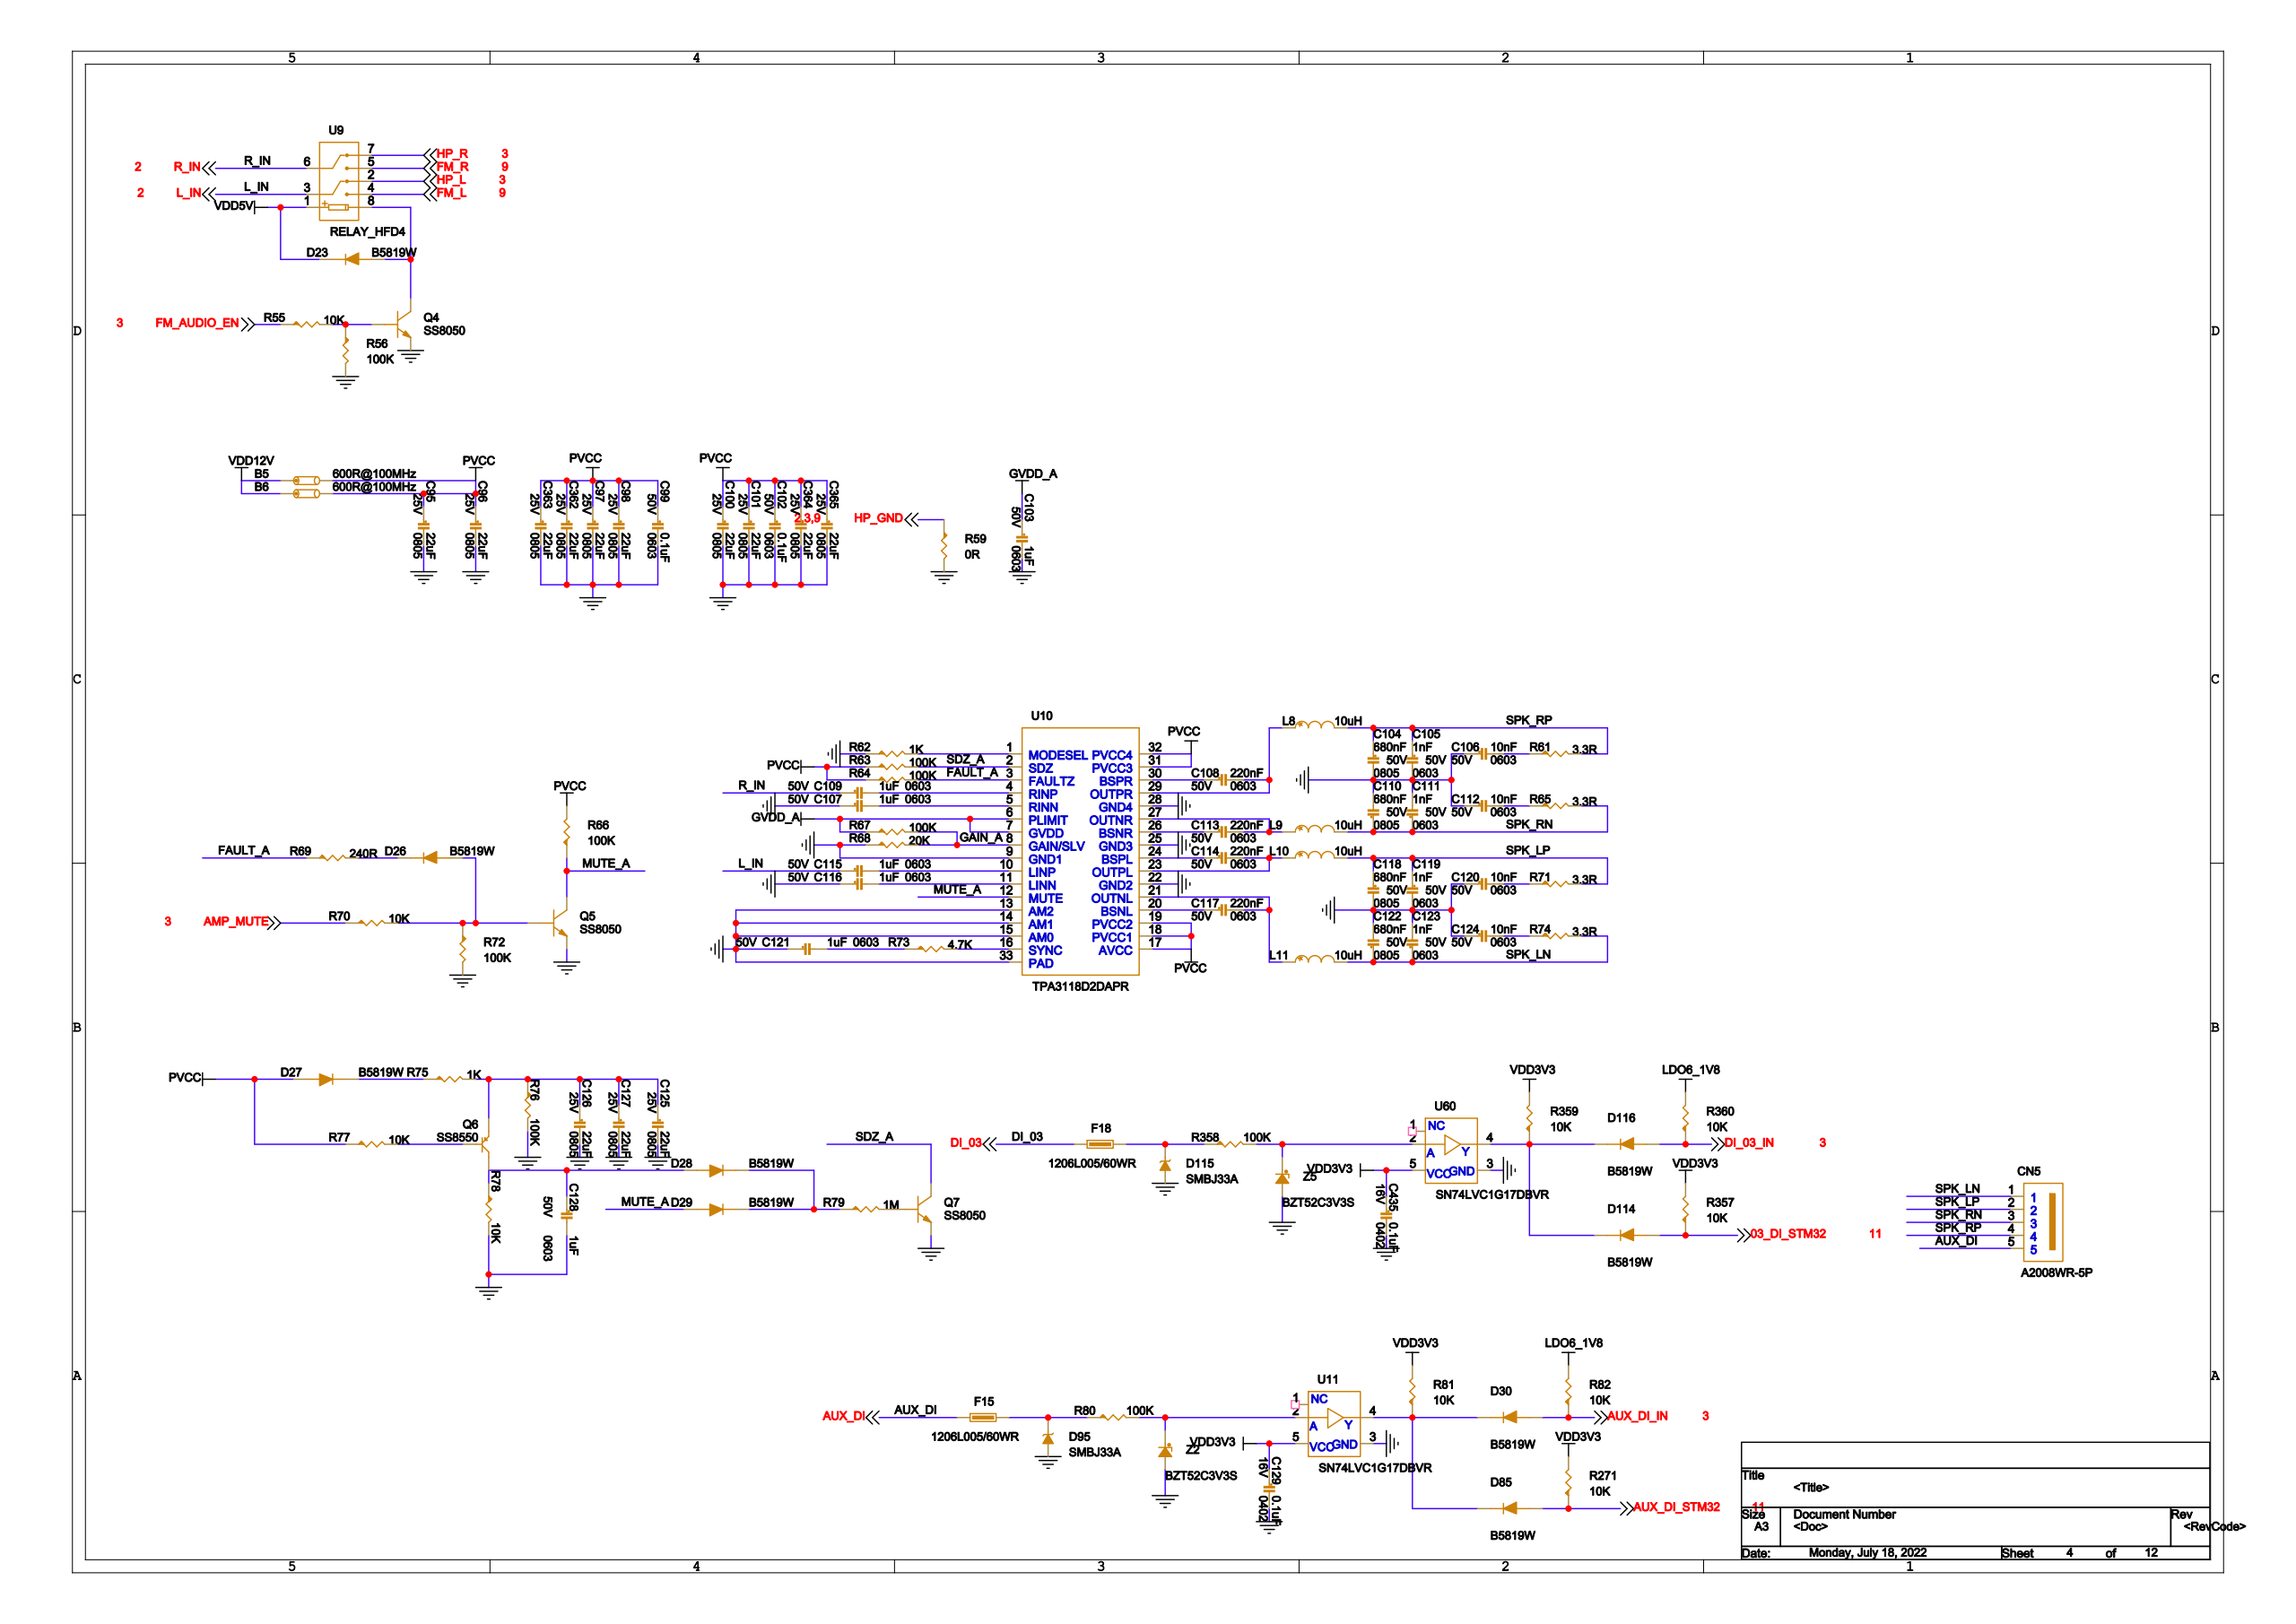Circuit board | Cadence Allegro | 970 parts | 627 nets | one sheet of the schematic
Parts on this sheet (reference | value | footprint):
B5 | 600R@100MHz | R0805
B6 | 600R@100MHz | R0805
C95 | 22uF | C0805
C96 | 22uF | C0805
C97 | 22uF | C0805
C98 | 22uF | C0805
C99 | 0.1uF | C0603
C100 | 22uF | C0805
C101 | 22uF | C0805
C102 | 0.1uF | C0603
C103 | 1uF | C0603
C104 | 680nF | C0805
C105 | 1nF | C0603
C106 | 10nF | C0603
C107 | 1uF | C0603
C108 | 220nF | C0603
C109 | 1uF | C0603
C110 | 680nF | C0805
C111 | 1nF | C0603
C112 | 10nF | C0603
C113 | 220nF | C0603
C114 | 220nF | C0603
C115 | 1uF | C0603
C116 | 1uF | C0603
C117 | 220nF | C0603
C118 | 680nF | C0805
C119 | 1nF | C0603
C120 | 10nF | C0603
C121 | 1uF | C0603
C122 | 680nF | C0805
C123 | 1nF | C0603
C124 | 10nF | C0603
C125 | 22uF | C0805
C126 | 22uF | C0805
C127 | 22uF | C0805
C128 | 1uF | C0603
C129 | 0.1uF | C0402
C362 | 22uF | C0805
C363 | 22uF | C0805
C364 | 22uF | C0805
C365 | 22uF | C0805
C435 | 0.1uF | C0402
CN5 | A2008WR-5P | A2008WR_5P
D23 | B5819W | SOD-123
D26 | B5819W | SOD-123
D27 | B5819W | SOD-123
D28 | B5819W | SOD-123
D29 | B5819W | SOD-123
D30 | B5819W | SOD-123
D85 | B5819W | SOD-123
D95 | SMBJ33A | SMB
D114 | B5819W | SOD-123
D115 | SMBJ33A | SMB
D116 | B5819W | SOD-123
F15 | 1206L005/60WR | R1206
F18 | 1206L005/60WR | R1206
L8 | 10uH | IND0630
L9 | 10uH | IND0630
L10 | 10uH | IND0630
L11 | 10uH | IND0630
Q4 | SS8050 | SOT-23
Q5 | SS8050 | SOT-23
Q6 | SS8550 | SOT-23
Q7 | SS8050 | SOT-23
R55 | 10K | R0402
R56 | 100K | R0402
R59 | 0R | R0402
R61 | 3.3R | R0603
R62 | 1K | R0402
R63 | 100K | R0402
R64 | 100K | R0402
R65 | 3.3R | R0603
R66 | 100K | R0402
R67 | 100K | R0402
R68 | 20K | R0402
R69 | 240R | R0402
R70 | 10K | R0402
R71 | 3.3R | R0603
R72 | 100K | R0402
R73 | 4.7K | R0402
R74 | 3.3R | R0603
R75 | 1K | R0402
R76 | 100K | R0402
R77 | 10K | R0402
R78 | 10K | R0402
R79 | 1M | R0402
R80 | 100K | R0402
R81 | 10K | R0402
R82 | 10K | R0402
R271 | 10K | R0402
R357 | 10K | R0402
R358 | 100K | R0402
R359 | 10K | R0402
R360 | 10K | R0402
U9 | RELAY_HFD4 | RELAY_HFD4
U10 | TPA3118D2DAPR | HTSSOP32
U11 | SN74LVC1G17DBVR | SOT23-5
U60 | SN74LVC1G17DBVR | SOT23-5
Z2 | BZT52C3V3S | SOD323
Z5 | BZT52C3V3S | SOD323
Nets of these parts (net: part-pin ...):
VDD5V: D23-2 U9-1
VDD3V3: C129-1 C435-1 R81-2 R271-2 R357-2 R359-2 U11-5 U60-5
GND: C95-2 C96-2 C97-2 C98-2 C99-2 C100-2 C101-2 C102-2 C103-2 C104-2 C105-2 C106-1 C107-1 C110-2 C111-2 C112-1 C116-1 C118-2 C119-2 C120-1 C121-1 C122-2 C123-2 C124-1 C125-2 C126-2 C127-2 C128-2 C129-2 C362-2 C363-2 C364-2 C365-2 C435-2 D95-1 D115-1 Q4-2 Q5-2 Q7-2 R56-2 R59-2 R62-1 R68-1 R72-2 R76-2 R78-2 U11-3 U60-3 Z2-1 Z5-1 U10-9 U10-13 U10-14 U10-15 U10-22 U10-25 U10-28 U10-33
LDO6_1V8: R82-2 R360-2
SPK_LN: C122-1 C123-1 CN5-1 L11-2 R74-2
SPK_LP: C118-1 C119-1 CN5-2 L10-2 R71-2
SPK_RN: C110-1 C111-1 CN5-3 L9-2 R65-2
SPK_RP: C104-1 C105-1 CN5-4 L8-2 R61-2
AUX_DI: CN5-5 F15-1
VDD12V: B5-1 B6-1
N19779625: D115-2 F18-2 R358-1
N19387563: D95-2 F15-2 R80-1
DI_03: F18-1
N19779643: R358-2 U60-2 Z5-2
N19779563: D114-2 D116-2 R359-1 U60-4
N19387544: R80-2 U11-2 Z2-2
N19387510: D30-2 D85-2 R81-1 U11-4
HP_L: U9-2
HP_GND: R59-1
HP_R: U9-7
N19224261: C106-2 R61-1
N19224258: C112-2 R65-1
N19224400: C120-2 R71-1
N19224398: C124-2 R74-1
N19223689: C108-1 U10-30
N19223692: C108-2 L8-1 U10-29
N19223701: C113-1 U10-26
N19223704: C113-2 L9-1 U10-27
N19223713: C114-1 U10-24
N19223716: C114-2 L10-1 U10-23
N19223725: C117-1 U10-20
N19223728: C117-2 L11-1 U10-21
R_IN: C109-1 U9-6
N19222303: C109-2 U10-4
N19222323: C107-2 U10-5
L_IN: C115-1 U9-3
N19222643: C115-2 U10-10
N19222646: C116-2 U10-11
N19222786: C121-2 R73-1
N19226459: C128-1 D28-1 Q6-3 R78-1
FM_L: U9-4
FM_R: U9-5
GVDD_A: C103-1 R67-1 U10-6 U10-7
PVCC: B5-2 B6-2 C95-1 C96-1 C97-1 C98-1 C99-1 C100-1 C101-1 C102-1 C362-1 C363-1 C364-1 C365-1 D27-1 R63-1 R64-1 R66-2 R77-1 U10-17 U10-18 U10-19 U10-31 U10-32
N19226387: C125-1 C126-1 C127-1 Q6-2 R75-2 R76-1
03_DI_STM32: D114-1 R357-1
DI_03_IN: D116-1 R360-1
AUX_DI_STM32: D85-1 R271-1
N19525361: D23-1 Q4-3 U9-8
N19224802: D26-1 Q5-1 R70-2 R72-1
N19224782: D26-2 R69-2
N19226369: D27-2 R75-1
N19228380: D28-2 D29-2 R79-1
MUTE_A: D29-1 Q5-3 R66-1 U10-12
AUX_DI_IN: D30-1 R82-1
N19219398: Q4-1 R55-2 R56-1
N192284141: Q7-1 R79-2
SDZ_A: Q7-3 R63-2 U10-2
N19226405: Q6-1 R77-2
FAULT_A: R64-2 R69-1 U10-3
GAIN_A: R67-2 R68-2 U10-8
N19222789: R73-2 U10-16
N19221923: R62-2 U10-1
FM_AUDIO_EN: R55-1
AMP_MUTE: R70-1